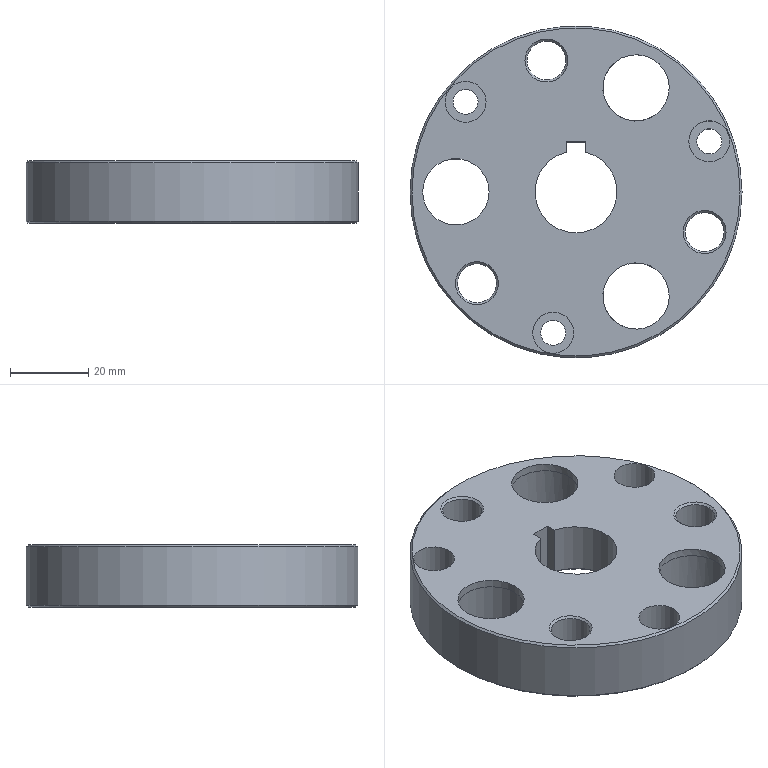Part | NX | features BREP 1 | 1 solid | 45 faces | box 85 x 85 x 16 mm | volume 64345 mm3 | cylinder 18 | cone 15 | plane 12 | commonest cylinder face diameters 6.4 x3 10 x3 10.5 x3 17 x3 19 x3 21 x1
STEP:
#1=CARTESIAN_POINT('',(25.38,26.639,0.));
#2=VERTEX_POINT('',#1);
#3=CARTESIAN_POINT('',(15.38,26.639,0.));
#4=DIRECTION('',(0.,0.,1.));
#5=DIRECTION('',(1.,0.,0.));
#6=AXIS2_PLACEMENT_3D('',#3,#4,#5);
#7=CIRCLE('',#6,10.);
#8=EDGE_CURVE('',#2,#2,#7,.T.);
#9=ORIENTED_EDGE('',*,*,#8,.F.);
#10=EDGE_LOOP('',(#9));
#11=FACE_BOUND('',#10,.T.);
#12=CARTESIAN_POINT('',(24.88,26.639,0.5));
#13=VERTEX_POINT('',#12);
#14=CARTESIAN_POINT('',(15.38,26.639,0.5));
#15=DIRECTION('',(0.,0.,-1.));
#16=DIRECTION('',(1.,0.,0.));
#17=AXIS2_PLACEMENT_3D('',#14,#15,#16);
#18=CIRCLE('',#17,9.5);
#19=EDGE_CURVE('',#13,#13,#18,.T.);
#20=ORIENTED_EDGE('',*,*,#19,.F.);
#21=EDGE_LOOP('',(#20));
#22=FACE_BOUND('',#21,.T.);
#23=CARTESIAN_POINT('',(15.38,26.639,0.));
#24=DIRECTION('',(0.,0.,-1.));
#25=DIRECTION('',(-1.,0.,0.));
#26=AXIS2_PLACEMENT_3D('',#23,#24,#25);
#27=CONICAL_SURFACE('',#26,10.,0.7854);
#28=ADVANCED_FACE('',(#11,#22),#27,.F.);
#29=CARTESIAN_POINT('',(25.38,-26.639,0.));
#30=VERTEX_POINT('',#29);
#31=CARTESIAN_POINT('',(15.38,-26.639,0.));
#32=DIRECTION('',(0.,0.,1.));
#33=DIRECTION('',(1.,0.,0.));
#34=AXIS2_PLACEMENT_3D('',#31,#32,#33);
#35=CIRCLE('',#34,10.);
#36=EDGE_CURVE('',#30,#30,#35,.T.);
#37=ORIENTED_EDGE('',*,*,#36,.F.);
#38=EDGE_LOOP('',(#37));
#39=FACE_BOUND('',#38,.T.);
#40=CARTESIAN_POINT('',(24.88,-26.639,0.5));
#41=VERTEX_POINT('',#40);
#42=CARTESIAN_POINT('',(15.38,-26.639,0.5));
#43=DIRECTION('',(0.,0.,-1.));
#44=DIRECTION('',(1.,0.,0.));
#45=AXIS2_PLACEMENT_3D('',#42,#43,#44);
#46=CIRCLE('',#45,9.5);
#47=EDGE_CURVE('',#41,#41,#46,.T.);
#48=ORIENTED_EDGE('',*,*,#47,.F.);
#49=EDGE_LOOP('',(#48));
#50=FACE_BOUND('',#49,.T.);
#51=CARTESIAN_POINT('',(15.38,-26.639,0.));
#52=DIRECTION('',(0.,0.,-1.));
#53=DIRECTION('',(-1.,0.,0.));
#54=AXIS2_PLACEMENT_3D('',#51,#52,#53);
#55=CONICAL_SURFACE('',#54,10.,0.7854);
#56=ADVANCED_FACE('',(#39,#50),#55,.F.);
#57=CARTESIAN_POINT('',(-20.76,0.,0.));
#58=VERTEX_POINT('',#57);
#59=CARTESIAN_POINT('',(-30.76,0.,0.));
#60=DIRECTION('',(0.,0.,1.));
#61=DIRECTION('',(1.,0.,0.));
#62=AXIS2_PLACEMENT_3D('',#59,#60,#61);
#63=CIRCLE('',#62,10.);
#64=EDGE_CURVE('',#58,#58,#63,.T.);
#65=ORIENTED_EDGE('',*,*,#64,.F.);
#66=EDGE_LOOP('',(#65));
#67=FACE_BOUND('',#66,.T.);
#68=CARTESIAN_POINT('',(-21.26,0.,0.5));
#69=VERTEX_POINT('',#68);
#70=CARTESIAN_POINT('',(-30.76,0.,0.5));
#71=DIRECTION('',(0.,0.,-1.));
#72=DIRECTION('',(1.,0.,0.));
#73=AXIS2_PLACEMENT_3D('',#70,#71,#72);
#74=CIRCLE('',#73,9.5);
#75=EDGE_CURVE('',#69,#69,#74,.T.);
#76=ORIENTED_EDGE('',*,*,#75,.F.);
#77=EDGE_LOOP('',(#76));
#78=FACE_BOUND('',#77,.T.);
#79=CARTESIAN_POINT('',(-30.76,0.,0.));
#80=DIRECTION('',(0.,0.,-1.));
#81=DIRECTION('',(-1.,0.,0.));
#82=AXIS2_PLACEMENT_3D('',#79,#80,#81);
#83=CONICAL_SURFACE('',#82,10.,0.7854);
#84=ADVANCED_FACE('',(#67,#78),#83,.F.);
#85=CARTESIAN_POINT('',(14.5,0.,0.));
#86=VERTEX_POINT('',#85);
#87=CARTESIAN_POINT('',(0.,0.,0.));
#88=DIRECTION('',(0.,0.,1.));
#89=DIRECTION('',(1.,0.,0.));
#90=AXIS2_PLACEMENT_3D('',#87,#88,#89);
#91=CIRCLE('',#90,14.5);
#92=EDGE_CURVE('',#86,#86,#91,.T.);
#93=ORIENTED_EDGE('',*,*,#92,.F.);
#94=EDGE_LOOP('',(#93));
#95=FACE_BOUND('',#94,.T.);
#96=CARTESIAN_POINT('',(14.,0.,0.5));
#97=VERTEX_POINT('',#96);
#98=CARTESIAN_POINT('',(0.,0.,0.5));
#99=DIRECTION('',(0.,0.,-1.));
#100=DIRECTION('',(1.,0.,0.));
#101=AXIS2_PLACEMENT_3D('',#98,#99,#100);
#102=CIRCLE('',#101,14.);
#103=EDGE_CURVE('',#97,#97,#102,.T.);
#104=ORIENTED_EDGE('',*,*,#103,.F.);
#105=EDGE_LOOP('',(#104));
#106=FACE_BOUND('',#105,.T.);
#107=CARTESIAN_POINT('',(0.,0.,0.5));
#108=DIRECTION('',(0.,0.,-1.));
#109=DIRECTION('',(-1.,0.,0.));
#110=AXIS2_PLACEMENT_3D('',#107,#108,#109);
#111=CONICAL_SURFACE('',#110,14.,0.7854);
#112=ADVANCED_FACE('',(#95,#106),#111,.F.);
#113=CARTESIAN_POINT('',(-23.029,23.076,16.));
#114=VERTEX_POINT('',#113);
#115=CARTESIAN_POINT('',(-28.279,23.076,16.));
#116=DIRECTION('',(0.,0.,1.));
#117=DIRECTION('',(1.,0.,0.));
#118=AXIS2_PLACEMENT_3D('',#115,#116,#117);
#119=CIRCLE('',#118,5.25);
#120=EDGE_CURVE('',#114,#114,#119,.T.);
#121=ORIENTED_EDGE('',*,*,#120,.T.);
#122=EDGE_LOOP('',(#121));
#123=FACE_BOUND('',#122,.T.);
#124=CARTESIAN_POINT('',(-23.029,23.076,8.5));
#125=VERTEX_POINT('',#124);
#126=CARTESIAN_POINT('',(-28.279,23.076,8.5));
#127=DIRECTION('',(0.,0.,1.));
#128=DIRECTION('',(1.,0.,0.));
#129=AXIS2_PLACEMENT_3D('',#126,#127,#128);
#130=CIRCLE('',#129,5.25);
#131=EDGE_CURVE('',#125,#125,#130,.T.);
#132=ORIENTED_EDGE('',*,*,#131,.F.);
#133=EDGE_LOOP('',(#132));
#134=FACE_BOUND('',#133,.T.);
#135=CARTESIAN_POINT('',(-28.279,23.076,16.));
#136=DIRECTION('',(0.,0.,1.));
#137=DIRECTION('',(1.,0.,0.));
#138=AXIS2_PLACEMENT_3D('',#135,#136,#137);
#139=CYLINDRICAL_SURFACE('',#138,5.25);
#140=ADVANCED_FACE('',(#123,#134),#139,.F.);
#141=CARTESIAN_POINT('',(39.375,12.952,16.));
#142=VERTEX_POINT('',#141);
#143=CARTESIAN_POINT('',(34.125,12.952,16.));
#144=DIRECTION('',(0.,0.,1.));
#145=DIRECTION('',(1.,0.,0.));
#146=AXIS2_PLACEMENT_3D('',#143,#144,#145);
#147=CIRCLE('',#146,5.25);
#148=EDGE_CURVE('',#142,#142,#147,.T.);
#149=ORIENTED_EDGE('',*,*,#148,.T.);
#150=EDGE_LOOP('',(#149));
#151=FACE_BOUND('',#150,.T.);
#152=CARTESIAN_POINT('',(39.375,12.952,8.5));
#153=VERTEX_POINT('',#152);
#154=CARTESIAN_POINT('',(34.125,12.952,8.5));
#155=DIRECTION('',(0.,0.,1.));
#156=DIRECTION('',(1.,0.,0.));
#157=AXIS2_PLACEMENT_3D('',#154,#155,#156);
#158=CIRCLE('',#157,5.25);
#159=EDGE_CURVE('',#153,#153,#158,.T.);
#160=ORIENTED_EDGE('',*,*,#159,.F.);
#161=EDGE_LOOP('',(#160));
#162=FACE_BOUND('',#161,.T.);
#163=CARTESIAN_POINT('',(34.125,12.952,16.));
#164=DIRECTION('',(0.,0.,1.));
#165=DIRECTION('',(1.,0.,0.));
#166=AXIS2_PLACEMENT_3D('',#163,#164,#165);
#167=CYLINDRICAL_SURFACE('',#166,5.25);
#168=ADVANCED_FACE('',(#151,#162),#167,.F.);
#169=CARTESIAN_POINT('',(-0.5951,-36.029,16.));
#170=VERTEX_POINT('',#169);
#171=CARTESIAN_POINT('',(-5.845,-36.029,16.));
#172=DIRECTION('',(0.,0.,1.));
#173=DIRECTION('',(1.,0.,0.));
#174=AXIS2_PLACEMENT_3D('',#171,#172,#173);
#175=CIRCLE('',#174,5.25);
#176=EDGE_CURVE('',#170,#170,#175,.T.);
#177=ORIENTED_EDGE('',*,*,#176,.T.);
#178=EDGE_LOOP('',(#177));
#179=FACE_BOUND('',#178,.T.);
#180=CARTESIAN_POINT('',(-0.5951,-36.029,8.5));
#181=VERTEX_POINT('',#180);
#182=CARTESIAN_POINT('',(-5.845,-36.029,8.5));
#183=DIRECTION('',(0.,0.,1.));
#184=DIRECTION('',(1.,0.,0.));
#185=AXIS2_PLACEMENT_3D('',#182,#183,#184);
#186=CIRCLE('',#185,5.25);
#187=EDGE_CURVE('',#181,#181,#186,.T.);
#188=ORIENTED_EDGE('',*,*,#187,.F.);
#189=EDGE_LOOP('',(#188));
#190=FACE_BOUND('',#189,.T.);
#191=CARTESIAN_POINT('',(-5.845,-36.029,16.));
#192=DIRECTION('',(0.,0.,1.));
#193=DIRECTION('',(1.,0.,0.));
#194=AXIS2_PLACEMENT_3D('',#191,#192,#193);
#195=CYLINDRICAL_SURFACE('',#194,5.25);
#196=ADVANCED_FACE('',(#179,#190),#195,.F.);
#197=ORIENTED_EDGE('',*,*,#103,.T.);
#198=EDGE_LOOP('',(#197));
#199=FACE_BOUND('',#198,.T.);
#200=CARTESIAN_POINT('',(-14.,0.,3.));
#201=VERTEX_POINT('',#200);
#202=CARTESIAN_POINT('',(0.,0.,3.));
#203=DIRECTION('',(0.,0.,-1.));
#204=DIRECTION('',(-1.,0.,0.));
#205=AXIS2_PLACEMENT_3D('',#202,#203,#204);
#206=CIRCLE('',#205,14.);
#207=EDGE_CURVE('',#201,#201,#206,.T.);
#208=ORIENTED_EDGE('',*,*,#207,.F.);
#209=EDGE_LOOP('',(#208));
#210=FACE_BOUND('',#209,.T.);
#211=CARTESIAN_POINT('',(0.,0.,3.));
#212=DIRECTION('',(0.,0.,-1.));
#213=DIRECTION('',(-1.,0.,0.));
#214=AXIS2_PLACEMENT_3D('',#211,#212,#213);
#215=CYLINDRICAL_SURFACE('',#214,14.);
#216=ADVANCED_FACE('',(#199,#210),#215,.F.);
#217=CARTESIAN_POINT('',(42.5,0.,15.5));
#218=VERTEX_POINT('',#217);
#219=CARTESIAN_POINT('',(0.,0.,15.5));
#220=DIRECTION('',(0.,0.,-1.));
#221=DIRECTION('',(1.,0.,0.));
#222=AXIS2_PLACEMENT_3D('',#219,#220,#221);
#223=CIRCLE('',#222,42.5);
#224=EDGE_CURVE('',#218,#218,#223,.T.);
#225=ORIENTED_EDGE('',*,*,#224,.F.);
#226=EDGE_LOOP('',(#225));
#227=FACE_BOUND('',#226,.T.);
#228=CARTESIAN_POINT('',(42.,0.,16.));
#229=VERTEX_POINT('',#228);
#230=CARTESIAN_POINT('',(0.,0.,16.));
#231=DIRECTION('',(0.,0.,1.));
#232=DIRECTION('',(1.,0.,0.));
#233=AXIS2_PLACEMENT_3D('',#230,#231,#232);
#234=CIRCLE('',#233,42.);
#235=EDGE_CURVE('',#229,#229,#234,.T.);
#236=ORIENTED_EDGE('',*,*,#235,.F.);
#237=EDGE_LOOP('',(#236));
#238=FACE_BOUND('',#237,.T.);
#239=CARTESIAN_POINT('',(0.,0.,16.));
#240=DIRECTION('',(0.,0.,-1.));
#241=DIRECTION('',(-1.,0.,0.));
#242=AXIS2_PLACEMENT_3D('',#239,#240,#241);
#243=CONICAL_SURFACE('',#242,42.,0.7854);
#244=ADVANCED_FACE('',(#227,#238),#243,.T.);
#245=CARTESIAN_POINT('',(42.5,0.,0.5));
#246=VERTEX_POINT('',#245);
#247=CARTESIAN_POINT('',(0.,0.,0.5));
#248=DIRECTION('',(0.,0.,1.));
#249=DIRECTION('',(1.,0.,0.));
#250=AXIS2_PLACEMENT_3D('',#247,#248,#249);
#251=CIRCLE('',#250,42.5);
#252=EDGE_CURVE('',#246,#246,#251,.T.);
#253=ORIENTED_EDGE('',*,*,#252,.F.);
#254=EDGE_LOOP('',(#253));
#255=FACE_BOUND('',#254,.T.);
#256=CARTESIAN_POINT('',(42.,0.,0.));
#257=VERTEX_POINT('',#256);
#258=CARTESIAN_POINT('',(0.,0.,0.));
#259=DIRECTION('',(0.,0.,-1.));
#260=DIRECTION('',(1.,0.,0.));
#261=AXIS2_PLACEMENT_3D('',#258,#259,#260);
#262=CIRCLE('',#261,42.);
#263=EDGE_CURVE('',#257,#257,#262,.T.);
#264=ORIENTED_EDGE('',*,*,#263,.F.);
#265=EDGE_LOOP('',(#264));
#266=FACE_BOUND('',#265,.T.);
#267=CARTESIAN_POINT('',(0.,0.,0.5));
#268=DIRECTION('',(0.,0.,1.));
#269=DIRECTION('',(1.,0.,0.));
#270=AXIS2_PLACEMENT_3D('',#267,#268,#269);
#271=CONICAL_SURFACE('',#270,42.5,0.7854);
#272=ADVANCED_FACE('',(#255,#266),#271,.T.);
#273=CARTESIAN_POINT('',(38.427,-10.265,16.));
#274=VERTEX_POINT('',#273);
#275=CARTESIAN_POINT('',(32.927,-10.265,16.));
#276=DIRECTION('',(0.,0.,-1.));
#277=DIRECTION('',(1.,0.,0.));
#278=AXIS2_PLACEMENT_3D('',#275,#276,#277);
#279=CIRCLE('',#278,5.5);
#280=EDGE_CURVE('',#274,#274,#279,.T.);
#281=ORIENTED_EDGE('',*,*,#280,.F.);
#282=EDGE_LOOP('',(#281));
#283=FACE_BOUND('',#282,.T.);
#284=CARTESIAN_POINT('',(37.927,-10.265,15.5));
#285=VERTEX_POINT('',#284);
#286=CARTESIAN_POINT('',(32.927,-10.265,15.5));
#287=DIRECTION('',(0.,0.,1.));
#288=DIRECTION('',(1.,0.,0.));
#289=AXIS2_PLACEMENT_3D('',#286,#287,#288);
#290=CIRCLE('',#289,5.);
#291=EDGE_CURVE('',#285,#285,#290,.T.);
#292=ORIENTED_EDGE('',*,*,#291,.F.);
#293=EDGE_LOOP('',(#292));
#294=FACE_BOUND('',#293,.T.);
#295=CARTESIAN_POINT('',(32.927,-10.265,16.));
#296=DIRECTION('',(0.,0.,1.));
#297=DIRECTION('',(1.,0.,0.));
#298=AXIS2_PLACEMENT_3D('',#295,#296,#297);
#299=CONICAL_SURFACE('',#298,5.5,0.7854);
#300=ADVANCED_FACE('',(#283,#294),#299,.F.);
#301=CARTESIAN_POINT('',(38.427,-10.265,0.));
#302=VERTEX_POINT('',#301);
#303=CARTESIAN_POINT('',(32.927,-10.265,0.));
#304=DIRECTION('',(0.,0.,1.));
#305=DIRECTION('',(1.,0.,0.));
#306=AXIS2_PLACEMENT_3D('',#303,#304,#305);
#307=CIRCLE('',#306,5.5);
#308=EDGE_CURVE('',#302,#302,#307,.T.);
#309=ORIENTED_EDGE('',*,*,#308,.F.);
#310=EDGE_LOOP('',(#309));
#311=FACE_BOUND('',#310,.T.);
#312=CARTESIAN_POINT('',(37.927,-10.265,0.5));
#313=VERTEX_POINT('',#312);
#314=CARTESIAN_POINT('',(32.927,-10.265,0.5));
#315=DIRECTION('',(0.,0.,-1.));
#316=DIRECTION('',(1.,0.,0.));
#317=AXIS2_PLACEMENT_3D('',#314,#315,#316);
#318=CIRCLE('',#317,5.);
#319=EDGE_CURVE('',#313,#313,#318,.T.);
#320=ORIENTED_EDGE('',*,*,#319,.F.);
#321=EDGE_LOOP('',(#320));
#322=FACE_BOUND('',#321,.T.);
#323=CARTESIAN_POINT('',(32.927,-10.265,0.5));
#324=DIRECTION('',(0.,0.,-1.));
#325=DIRECTION('',(-1.,0.,0.));
#326=AXIS2_PLACEMENT_3D('',#323,#324,#325);
#327=CONICAL_SURFACE('',#326,5.,0.7854);
#328=ADVANCED_FACE('',(#311,#322),#327,.F.);
#329=CARTESIAN_POINT('',(37.825,12.952,0.));
#330=VERTEX_POINT('',#329);
#331=CARTESIAN_POINT('',(34.125,12.952,0.));
#332=DIRECTION('',(0.,0.,1.));
#333=DIRECTION('',(1.,0.,0.));
#334=AXIS2_PLACEMENT_3D('',#331,#332,#333);
#335=CIRCLE('',#334,3.7);
#336=EDGE_CURVE('',#330,#330,#335,.T.);
#337=ORIENTED_EDGE('',*,*,#336,.F.);
#338=EDGE_LOOP('',(#337));
#339=FACE_BOUND('',#338,.T.);
#340=CARTESIAN_POINT('',(37.325,12.952,0.5));
#341=VERTEX_POINT('',#340);
#342=CARTESIAN_POINT('',(34.125,12.952,0.5));
#343=DIRECTION('',(0.,0.,-1.));
#344=DIRECTION('',(1.,0.,0.));
#345=AXIS2_PLACEMENT_3D('',#342,#343,#344);
#346=CIRCLE('',#345,3.2);
#347=EDGE_CURVE('',#341,#341,#346,.T.);
#348=ORIENTED_EDGE('',*,*,#347,.F.);
#349=EDGE_LOOP('',(#348));
#350=FACE_BOUND('',#349,.T.);
#351=CARTESIAN_POINT('',(34.125,12.952,0.5));
#352=DIRECTION('',(0.,0.,-1.));
#353=DIRECTION('',(-1.,0.,0.));
#354=AXIS2_PLACEMENT_3D('',#351,#352,#353);
#355=CONICAL_SURFACE('',#354,3.2,0.7854);
#356=ADVANCED_FACE('',(#339,#350),#355,.F.);
#357=CARTESIAN_POINT('',(-2.074,33.648,16.));
#358=VERTEX_POINT('',#357);
#359=CARTESIAN_POINT('',(-7.574,33.648,16.));
#360=DIRECTION('',(0.,0.,-1.));
#361=DIRECTION('',(1.,0.,0.));
#362=AXIS2_PLACEMENT_3D('',#359,#360,#361);
#363=CIRCLE('',#362,5.5);
#364=EDGE_CURVE('',#358,#358,#363,.T.);
#365=ORIENTED_EDGE('',*,*,#364,.F.);
#366=EDGE_LOOP('',(#365));
#367=FACE_BOUND('',#366,.T.);
#368=CARTESIAN_POINT('',(-2.574,33.648,15.5));
#369=VERTEX_POINT('',#368);
#370=CARTESIAN_POINT('',(-7.574,33.648,15.5));
#371=DIRECTION('',(0.,0.,1.));
#372=DIRECTION('',(1.,0.,0.));
#373=AXIS2_PLACEMENT_3D('',#370,#371,#372);
#374=CIRCLE('',#373,5.);
#375=EDGE_CURVE('',#369,#369,#374,.T.);
#376=ORIENTED_EDGE('',*,*,#375,.F.);
#377=EDGE_LOOP('',(#376));
#378=FACE_BOUND('',#377,.T.);
#379=CARTESIAN_POINT('',(-7.574,33.648,16.));
#380=DIRECTION('',(0.,0.,1.));
#381=DIRECTION('',(1.,0.,0.));
#382=AXIS2_PLACEMENT_3D('',#379,#380,#381);
#383=CONICAL_SURFACE('',#382,5.5,0.7854);
#384=ADVANCED_FACE('',(#367,#378),#383,.F.);
#385=CARTESIAN_POINT('',(-2.074,33.648,0.));
#386=VERTEX_POINT('',#385);
#387=CARTESIAN_POINT('',(-7.574,33.648,0.));
#388=DIRECTION('',(0.,0.,1.));
#389=DIRECTION('',(1.,0.,0.));
#390=AXIS2_PLACEMENT_3D('',#387,#388,#389);
#391=CIRCLE('',#390,5.5);
#392=EDGE_CURVE('',#386,#386,#391,.T.);
#393=ORIENTED_EDGE('',*,*,#392,.F.);
#394=EDGE_LOOP('',(#393));
#395=FACE_BOUND('',#394,.T.);
#396=CARTESIAN_POINT('',(-2.574,33.648,0.5));
#397=VERTEX_POINT('',#396);
#398=CARTESIAN_POINT('',(-7.574,33.648,0.5));
#399=DIRECTION('',(0.,0.,-1.));
#400=DIRECTION('',(1.,0.,0.));
#401=AXIS2_PLACEMENT_3D('',#398,#399,#400);
#402=CIRCLE('',#401,5.);
#403=EDGE_CURVE('',#397,#397,#402,.T.);
#404=ORIENTED_EDGE('',*,*,#403,.F.);
#405=EDGE_LOOP('',(#404));
#406=FACE_BOUND('',#405,.T.);
#407=CARTESIAN_POINT('',(-7.574,33.648,0.5));
#408=DIRECTION('',(0.,0.,-1.));
#409=DIRECTION('',(-1.,0.,0.));
#410=AXIS2_PLACEMENT_3D('',#407,#408,#409);
#411=CONICAL_SURFACE('',#410,5.,0.7854);
#412=ADVANCED_FACE('',(#395,#406),#411,.F.);
#413=CARTESIAN_POINT('',(-24.579,23.076,0.));
#414=VERTEX_POINT('',#413);
#415=CARTESIAN_POINT('',(-28.279,23.076,0.));
#416=DIRECTION('',(0.,0.,1.));
#417=DIRECTION('',(1.,0.,0.));
#418=AXIS2_PLACEMENT_3D('',#415,#416,#417);
#419=CIRCLE('',#418,3.7);
#420=EDGE_CURVE('',#414,#414,#419,.T.);
#421=ORIENTED_EDGE('',*,*,#420,.F.);
#422=EDGE_LOOP('',(#421));
#423=FACE_BOUND('',#422,.T.);
#424=CARTESIAN_POINT('',(-25.079,23.076,0.5));
#425=VERTEX_POINT('',#424);
#426=CARTESIAN_POINT('',(-28.279,23.076,0.5));
#427=DIRECTION('',(0.,0.,-1.));
#428=DIRECTION('',(1.,0.,0.));
#429=AXIS2_PLACEMENT_3D('',#426,#427,#428);
#430=CIRCLE('',#429,3.2);
#431=EDGE_CURVE('',#425,#425,#430,.T.);
#432=ORIENTED_EDGE('',*,*,#431,.F.);
#433=EDGE_LOOP('',(#432));
#434=FACE_BOUND('',#433,.T.);
#435=CARTESIAN_POINT('',(-28.279,23.076,0.5));
#436=DIRECTION('',(0.,0.,-1.));
#437=DIRECTION('',(-1.,0.,0.));
#438=AXIS2_PLACEMENT_3D('',#435,#436,#437);
#439=CONICAL_SURFACE('',#438,3.2,0.7854);
#440=ADVANCED_FACE('',(#423,#434),#439,.F.);
#441=ORIENTED_EDGE('',*,*,#47,.T.);
#442=EDGE_LOOP('',(#441));
#443=FACE_BOUND('',#442,.T.);
#444=CARTESIAN_POINT('',(10.63,-18.412,14.));
#445=VERTEX_POINT('',#444);
#446=CARTESIAN_POINT('',(15.38,-26.639,14.));
#447=DIRECTION('',(0.,0.,1.));
#448=DIRECTION('',(-0.5,0.866,0.));
#449=AXIS2_PLACEMENT_3D('',#446,#447,#448);
#450=CIRCLE('',#449,9.5);
#451=EDGE_CURVE('',#445,#445,#450,.T.);
#452=ORIENTED_EDGE('',*,*,#451,.T.);
#453=EDGE_LOOP('',(#452));
#454=FACE_BOUND('',#453,.T.);
#455=CARTESIAN_POINT('',(15.38,-26.639,14.));
#456=DIRECTION('',(0.,0.,-1.));
#457=DIRECTION('',(-1.,0.,0.));
#458=AXIS2_PLACEMENT_3D('',#455,#456,#457);
#459=CYLINDRICAL_SURFACE('',#458,9.5);
#460=ADVANCED_FACE('',(#443,#454),#459,.F.);
#461=ORIENTED_EDGE('',*,*,#19,.T.);
#462=EDGE_LOOP('',(#461));
#463=FACE_BOUND('',#462,.T.);
#464=CARTESIAN_POINT('',(10.63,18.412,14.));
#465=VERTEX_POINT('',#464);
#466=CARTESIAN_POINT('',(15.38,26.639,14.));
#467=DIRECTION('',(0.,0.,1.));
#468=DIRECTION('',(-0.5,-0.866,0.));
#469=AXIS2_PLACEMENT_3D('',#466,#467,#468);
#470=CIRCLE('',#469,9.5);
#471=EDGE_CURVE('',#465,#465,#470,.T.);
#472=ORIENTED_EDGE('',*,*,#471,.T.);
#473=EDGE_LOOP('',(#472));
#474=FACE_BOUND('',#473,.T.);
#475=CARTESIAN_POINT('',(15.38,26.639,14.));
#476=DIRECTION('',(0.,0.,-1.));
#477=DIRECTION('',(-1.,0.,0.));
#478=AXIS2_PLACEMENT_3D('',#475,#476,#477);
#479=CYLINDRICAL_SURFACE('',#478,9.5);
#480=ADVANCED_FACE('',(#463,#474),#479,.F.);
#481=ORIENTED_EDGE('',*,*,#347,.T.);
#482=EDGE_LOOP('',(#481));
#483=FACE_BOUND('',#482,.T.);
#484=CARTESIAN_POINT('',(37.325,12.952,8.5));
#485=VERTEX_POINT('',#484);
#486=CARTESIAN_POINT('',(34.125,12.952,8.5));
#487=DIRECTION('',(0.,0.,1.));
#488=DIRECTION('',(1.,0.,0.));
#489=AXIS2_PLACEMENT_3D('',#486,#487,#488);
#490=CIRCLE('',#489,3.2);
#491=EDGE_CURVE('',#485,#485,#490,.T.);
#492=ORIENTED_EDGE('',*,*,#491,.T.);
#493=EDGE_LOOP('',(#492));
#494=FACE_BOUND('',#493,.T.);
#495=CARTESIAN_POINT('',(34.125,12.952,16.));
#496=DIRECTION('',(0.,0.,-1.));
#497=DIRECTION('',(-1.,0.,0.));
#498=AXIS2_PLACEMENT_3D('',#495,#496,#497);
#499=CYLINDRICAL_SURFACE('',#498,3.2);
#500=ADVANCED_FACE('',(#483,#494),#499,.F.);
#501=ORIENTED_EDGE('',*,*,#319,.T.);
#502=EDGE_LOOP('',(#501));
#503=FACE_BOUND('',#502,.T.);
#504=ORIENTED_EDGE('',*,*,#291,.T.);
#505=EDGE_LOOP('',(#504));
#506=FACE_BOUND('',#505,.T.);
#507=CARTESIAN_POINT('',(32.927,-10.265,16.));
#508=DIRECTION('',(0.,0.,-1.));
#509=DIRECTION('',(-1.,0.,0.));
#510=AXIS2_PLACEMENT_3D('',#507,#508,#509);
#511=CYLINDRICAL_SURFACE('',#510,5.);
#512=ADVANCED_FACE('',(#503,#506),#511,.F.);
#513=CARTESIAN_POINT('',(23.88,-26.639,14.));
#514=VERTEX_POINT('',#513);
#515=CARTESIAN_POINT('',(15.38,-26.639,14.));
#516=DIRECTION('',(0.,0.,-1.));
#517=DIRECTION('',(1.,0.,0.));
#518=AXIS2_PLACEMENT_3D('',#515,#516,#517);
#519=CIRCLE('',#518,8.5);
#520=EDGE_CURVE('',#514,#514,#519,.T.);
#521=ORIENTED_EDGE('',*,*,#520,.T.);
#522=EDGE_LOOP('',(#521));
#523=FACE_BOUND('',#522,.T.);
#524=CARTESIAN_POINT('',(19.63,-34.,16.));
#525=VERTEX_POINT('',#524);
#526=CARTESIAN_POINT('',(15.38,-26.639,16.));
#527=DIRECTION('',(0.,0.,-1.));
#528=DIRECTION('',(0.5,-0.866,0.));
#529=AXIS2_PLACEMENT_3D('',#526,#527,#528);
#530=CIRCLE('',#529,8.5);
#531=EDGE_CURVE('',#525,#525,#530,.T.);
#532=ORIENTED_EDGE('',*,*,#531,.F.);
#533=EDGE_LOOP('',(#532));
#534=FACE_BOUND('',#533,.T.);
#535=CARTESIAN_POINT('',(15.38,-26.639,16.));
#536=DIRECTION('',(0.,0.,-1.));
#537=DIRECTION('',(-1.,0.,0.));
#538=AXIS2_PLACEMENT_3D('',#535,#536,#537);
#539=CYLINDRICAL_SURFACE('',#538,8.5);
#540=ADVANCED_FACE('',(#523,#534),#539,.F.);
#541=ORIENTED_EDGE('',*,*,#431,.T.);
#542=EDGE_LOOP('',(#541));
#543=FACE_BOUND('',#542,.T.);
#544=CARTESIAN_POINT('',(-25.079,23.076,8.5));
#545=VERTEX_POINT('',#544);
#546=CARTESIAN_POINT('',(-28.279,23.076,8.5));
#547=DIRECTION('',(0.,0.,1.));
#548=DIRECTION('',(1.,0.,0.));
#549=AXIS2_PLACEMENT_3D('',#546,#547,#548);
#550=CIRCLE('',#549,3.2);
#551=EDGE_CURVE('',#545,#545,#550,.T.);
#552=ORIENTED_EDGE('',*,*,#551,.T.);
#553=EDGE_LOOP('',(#552));
#554=FACE_BOUND('',#553,.T.);
#555=CARTESIAN_POINT('',(-28.279,23.076,16.));
#556=DIRECTION('',(0.,0.,-1.));
#557=DIRECTION('',(-1.,0.,0.));
#558=AXIS2_PLACEMENT_3D('',#555,#556,#557);
#559=CYLINDRICAL_SURFACE('',#558,3.2);
#560=ADVANCED_FACE('',(#543,#554),#559,.F.);
#561=ORIENTED_EDGE('',*,*,#403,.T.);
#562=EDGE_LOOP('',(#561));
#563=FACE_BOUND('',#562,.T.);
#564=ORIENTED_EDGE('',*,*,#375,.T.);
#565=EDGE_LOOP('',(#564));
#566=FACE_BOUND('',#565,.T.);
#567=CARTESIAN_POINT('',(-7.574,33.648,16.));
#568=DIRECTION('',(0.,0.,-1.));
#569=DIRECTION('',(-1.,0.,0.));
#570=AXIS2_PLACEMENT_3D('',#567,#568,#569);
#571=CYLINDRICAL_SURFACE('',#570,5.);
#572=ADVANCED_FACE('',(#563,#566),#571,.F.);
#573=CARTESIAN_POINT('',(23.88,26.639,14.));
#574=VERTEX_POINT('',#573);
#575=CARTESIAN_POINT('',(15.38,26.639,14.));
#576=DIRECTION('',(0.,0.,-1.));
#577=DIRECTION('',(1.,0.,0.));
#578=AXIS2_PLACEMENT_3D('',#575,#576,#577);
#579=CIRCLE('',#578,8.5);
#580=EDGE_CURVE('',#574,#574,#579,.T.);
#581=ORIENTED_EDGE('',*,*,#580,.T.);
#582=EDGE_LOOP('',(#581));
#583=FACE_BOUND('',#582,.T.);
#584=CARTESIAN_POINT('',(19.63,34.,16.));
#585=VERTEX_POINT('',#584);
#586=CARTESIAN_POINT('',(15.38,26.639,16.));
#587=DIRECTION('',(0.,0.,-1.));
#588=DIRECTION('',(0.5,0.866,0.));
#589=AXIS2_PLACEMENT_3D('',#586,#587,#588);
#590=CIRCLE('',#589,8.5);
#591=EDGE_CURVE('',#585,#585,#590,.T.);
#592=ORIENTED_EDGE('',*,*,#591,.F.);
#593=EDGE_LOOP('',(#592));
#594=FACE_BOUND('',#593,.T.);
#595=CARTESIAN_POINT('',(15.38,26.639,16.));
#596=DIRECTION('',(0.,0.,-1.));
#597=DIRECTION('',(-1.,0.,0.));
#598=AXIS2_PLACEMENT_3D('',#595,#596,#597);
#599=CYLINDRICAL_SURFACE('',#598,8.5);
#600=ADVANCED_FACE('',(#583,#594),#599,.F.);
#601=CARTESIAN_POINT('',(-19.853,-23.383,16.));
#602=VERTEX_POINT('',#601);
#603=CARTESIAN_POINT('',(-25.353,-23.383,16.));
#604=DIRECTION('',(0.,0.,-1.));
#605=DIRECTION('',(1.,0.,0.));
#606=AXIS2_PLACEMENT_3D('',#603,#604,#605);
#607=CIRCLE('',#606,5.5);
#608=EDGE_CURVE('',#602,#602,#607,.T.);
#609=ORIENTED_EDGE('',*,*,#608,.F.);
#610=EDGE_LOOP('',(#609));
#611=FACE_BOUND('',#610,.T.);
#612=CARTESIAN_POINT('',(-20.353,-23.383,15.5));
#613=VERTEX_POINT('',#612);
#614=CARTESIAN_POINT('',(-25.353,-23.383,15.5));
#615=DIRECTION('',(0.,0.,1.));
#616=DIRECTION('',(1.,0.,0.));
#617=AXIS2_PLACEMENT_3D('',#614,#615,#616);
#618=CIRCLE('',#617,5.);
#619=EDGE_CURVE('',#613,#613,#618,.T.);
#620=ORIENTED_EDGE('',*,*,#619,.F.);
#621=EDGE_LOOP('',(#620));
#622=FACE_BOUND('',#621,.T.);
#623=CARTESIAN_POINT('',(-25.353,-23.383,16.));
#624=DIRECTION('',(0.,0.,1.));
#625=DIRECTION('',(1.,0.,0.));
#626=AXIS2_PLACEMENT_3D('',#623,#624,#625);
#627=CONICAL_SURFACE('',#626,5.5,0.7854);
#628=ADVANCED_FACE('',(#611,#622),#627,.F.);
#629=CARTESIAN_POINT('',(-19.853,-23.383,0.));
#630=VERTEX_POINT('',#629);
#631=CARTESIAN_POINT('',(-25.353,-23.383,0.));
#632=DIRECTION('',(0.,0.,1.));
#633=DIRECTION('',(1.,0.,0.));
#634=AXIS2_PLACEMENT_3D('',#631,#632,#633);
#635=CIRCLE('',#634,5.5);
#636=EDGE_CURVE('',#630,#630,#635,.T.);
#637=ORIENTED_EDGE('',*,*,#636,.F.);
#638=EDGE_LOOP('',(#637));
#639=FACE_BOUND('',#638,.T.);
#640=CARTESIAN_POINT('',(-20.353,-23.383,0.5));
#641=VERTEX_POINT('',#640);
#642=CARTESIAN_POINT('',(-25.353,-23.383,0.5));
#643=DIRECTION('',(0.,0.,-1.));
#644=DIRECTION('',(1.,0.,0.));
#645=AXIS2_PLACEMENT_3D('',#642,#643,#644);
#646=CIRCLE('',#645,5.);
#647=EDGE_CURVE('',#641,#641,#646,.T.);
#648=ORIENTED_EDGE('',*,*,#647,.F.);
#649=EDGE_LOOP('',(#648));
#650=FACE_BOUND('',#649,.T.);
#651=CARTESIAN_POINT('',(-25.353,-23.383,0.5));
#652=DIRECTION('',(0.,0.,-1.));
#653=DIRECTION('',(-1.,0.,0.));
#654=AXIS2_PLACEMENT_3D('',#651,#652,#653);
#655=CONICAL_SURFACE('',#654,5.,0.7854);
#656=ADVANCED_FACE('',(#639,#650),#655,.F.);
#657=CARTESIAN_POINT('',(-2.145,-36.029,0.));
#658=VERTEX_POINT('',#657);
#659=CARTESIAN_POINT('',(-5.845,-36.029,0.));
#660=DIRECTION('',(0.,0.,1.));
#661=DIRECTION('',(1.,0.,0.));
#662=AXIS2_PLACEMENT_3D('',#659,#660,#661);
#663=CIRCLE('',#662,3.7);
#664=EDGE_CURVE('',#658,#658,#663,.T.);
#665=ORIENTED_EDGE('',*,*,#664,.F.);
#666=EDGE_LOOP('',(#665));
#667=FACE_BOUND('',#666,.T.);
#668=CARTESIAN_POINT('',(-2.645,-36.029,0.5));
#669=VERTEX_POINT('',#668);
#670=CARTESIAN_POINT('',(-5.845,-36.029,0.5));
#671=DIRECTION('',(0.,0.,-1.));
#672=DIRECTION('',(1.,0.,0.));
#673=AXIS2_PLACEMENT_3D('',#670,#671,#672);
#674=CIRCLE('',#673,3.2);
#675=EDGE_CURVE('',#669,#669,#674,.T.);
#676=ORIENTED_EDGE('',*,*,#675,.F.);
#677=EDGE_LOOP('',(#676));
#678=FACE_BOUND('',#677,.T.);
#679=CARTESIAN_POINT('',(-5.845,-36.029,0.5));
#680=DIRECTION('',(0.,0.,-1.));
#681=DIRECTION('',(-1.,0.,0.));
#682=AXIS2_PLACEMENT_3D('',#679,#680,#681);
#683=CONICAL_SURFACE('',#682,3.2,0.7854);
#684=ADVANCED_FACE('',(#667,#678),#683,.F.);
#685=ORIENTED_EDGE('',*,*,#75,.T.);
#686=EDGE_LOOP('',(#685));
#687=FACE_BOUND('',#686,.T.);
#688=CARTESIAN_POINT('',(-21.26,0.,14.));
#689=VERTEX_POINT('',#688);
#690=CARTESIAN_POINT('',(-30.76,0.,14.));
#691=DIRECTION('',(0.,0.,1.));
#692=DIRECTION('',(1.,0.,0.));
#693=AXIS2_PLACEMENT_3D('',#690,#691,#692);
#694=CIRCLE('',#693,9.5);
#695=EDGE_CURVE('',#689,#689,#694,.T.);
#696=ORIENTED_EDGE('',*,*,#695,.T.);
#697=EDGE_LOOP('',(#696));
#698=FACE_BOUND('',#697,.T.);
#699=CARTESIAN_POINT('',(-30.76,0.,14.));
#700=DIRECTION('',(0.,0.,-1.));
#701=DIRECTION('',(-1.,0.,0.));
#702=AXIS2_PLACEMENT_3D('',#699,#700,#701);
#703=CYLINDRICAL_SURFACE('',#702,9.5);
#704=ADVANCED_FACE('',(#687,#698),#703,.F.);
#705=ORIENTED_EDGE('',*,*,#675,.T.);
#706=EDGE_LOOP('',(#705));
#707=FACE_BOUND('',#706,.T.);
#708=CARTESIAN_POINT('',(-2.645,-36.029,8.5));
#709=VERTEX_POINT('',#708);
#710=CARTESIAN_POINT('',(-5.845,-36.029,8.5));
#711=DIRECTION('',(0.,0.,1.));
#712=DIRECTION('',(1.,0.,0.));
#713=AXIS2_PLACEMENT_3D('',#710,#711,#712);
#714=CIRCLE('',#713,3.2);
#715=EDGE_CURVE('',#709,#709,#714,.T.);
#716=ORIENTED_EDGE('',*,*,#715,.T.);
#717=EDGE_LOOP('',(#716));
#718=FACE_BOUND('',#717,.T.);
#719=CARTESIAN_POINT('',(-5.845,-36.029,16.));
#720=DIRECTION('',(0.,0.,-1.));
#721=DIRECTION('',(-1.,0.,0.));
#722=AXIS2_PLACEMENT_3D('',#719,#720,#721);
#723=CYLINDRICAL_SURFACE('',#722,3.2);
#724=ADVANCED_FACE('',(#707,#718),#723,.F.);
#725=ORIENTED_EDGE('',*,*,#647,.T.);
#726=EDGE_LOOP('',(#725));
#727=FACE_BOUND('',#726,.T.);
#728=ORIENTED_EDGE('',*,*,#619,.T.);
#729=EDGE_LOOP('',(#728));
#730=FACE_BOUND('',#729,.T.);
#731=CARTESIAN_POINT('',(-25.353,-23.383,16.));
#732=DIRECTION('',(0.,0.,-1.));
#733=DIRECTION('',(-1.,0.,0.));
#734=AXIS2_PLACEMENT_3D('',#731,#732,#733);
#735=CYLINDRICAL_SURFACE('',#734,5.);
#736=ADVANCED_FACE('',(#727,#730),#735,.F.);
#737=CARTESIAN_POINT('',(-22.26,0.,14.));
#738=VERTEX_POINT('',#737);
#739=CARTESIAN_POINT('',(-30.76,0.,14.));
#740=DIRECTION('',(0.,0.,-1.));
#741=DIRECTION('',(1.,0.,0.));
#742=AXIS2_PLACEMENT_3D('',#739,#740,#741);
#743=CIRCLE('',#742,8.5);
#744=EDGE_CURVE('',#738,#738,#743,.T.);
#745=ORIENTED_EDGE('',*,*,#744,.T.);
#746=EDGE_LOOP('',(#745));
#747=FACE_BOUND('',#746,.T.);
#748=CARTESIAN_POINT('',(-39.26,0.,16.));
#749=VERTEX_POINT('',#748);
#750=CARTESIAN_POINT('',(-30.76,0.,16.));
#751=DIRECTION('',(0.,0.,-1.));
#752=DIRECTION('',(-1.,0.,0.));
#753=AXIS2_PLACEMENT_3D('',#750,#751,#752);
#754=CIRCLE('',#753,8.5);
#755=EDGE_CURVE('',#749,#749,#754,.T.);
#756=ORIENTED_EDGE('',*,*,#755,.F.);
#757=EDGE_LOOP('',(#756));
#758=FACE_BOUND('',#757,.T.);
#759=CARTESIAN_POINT('',(-30.76,0.,16.));
#760=DIRECTION('',(0.,0.,-1.));
#761=DIRECTION('',(-1.,0.,0.));
#762=AXIS2_PLACEMENT_3D('',#759,#760,#761);
#763=CYLINDRICAL_SURFACE('',#762,8.5);
#764=ADVANCED_FACE('',(#747,#758),#763,.F.);
#765=ORIENTED_EDGE('',*,*,#252,.T.);
#766=EDGE_LOOP('',(#765));
#767=FACE_BOUND('',#766,.T.);
#768=ORIENTED_EDGE('',*,*,#224,.T.);
#769=EDGE_LOOP('',(#768));
#770=FACE_BOUND('',#769,.T.);
#771=CARTESIAN_POINT('',(0.,0.,16.));
#772=DIRECTION('',(0.,0.,-1.));
#773=DIRECTION('',(-1.,0.,0.));
#774=AXIS2_PLACEMENT_3D('',#771,#772,#773);
#775=CYLINDRICAL_SURFACE('',#774,42.5);
#776=ADVANCED_FACE('',(#767,#770),#775,.T.);
#777=CARTESIAN_POINT('',(-2.5,10.198,16.));
#778=VERTEX_POINT('',#777);
#779=CARTESIAN_POINT('',(2.5,10.198,16.));
#780=VERTEX_POINT('',#779);
#781=CARTESIAN_POINT('',(0.,0.,16.));
#782=DIRECTION('',(0.,0.,1.));
#783=DIRECTION('',(1.,0.,0.));
#784=AXIS2_PLACEMENT_3D('',#781,#782,#783);
#785=CIRCLE('',#784,10.5);
#786=EDGE_CURVE('',#778,#780,#785,.T.);
#787=ORIENTED_EDGE('',*,*,#786,.T.);
#788=CARTESIAN_POINT('',(2.5,10.198,3.));
#789=VERTEX_POINT('',#788);
#790=CARTESIAN_POINT('',(2.5,10.198,16.));
#791=DIRECTION('',(0.,0.,-1.));
#792=VECTOR('',#791,1000.);
#793=LINE('',#790,#792);
#794=EDGE_CURVE('',#780,#789,#793,.T.);
#795=ORIENTED_EDGE('',*,*,#794,.T.);
#796=CARTESIAN_POINT('',(-2.5,10.198,3.));
#797=VERTEX_POINT('',#796);
#798=CARTESIAN_POINT('',(0.,0.,3.));
#799=DIRECTION('',(0.,0.,-1.));
#800=DIRECTION('',(-1.,0.,0.));
#801=AXIS2_PLACEMENT_3D('',#798,#799,#800);
#802=CIRCLE('',#801,10.5);
#803=EDGE_CURVE('',#789,#797,#802,.T.);
#804=ORIENTED_EDGE('',*,*,#803,.T.);
#805=CARTESIAN_POINT('',(-2.5,10.198,16.));
#806=DIRECTION('',(0.,0.,-1.));
#807=VECTOR('',#806,1000.);
#808=LINE('',#805,#807);
#809=EDGE_CURVE('',#778,#797,#808,.T.);
#810=ORIENTED_EDGE('',*,*,#809,.F.);
#811=EDGE_LOOP('',(#787,#795,#804,#810));
#812=FACE_BOUND('',#811,.T.);
#813=CARTESIAN_POINT('',(0.,0.,16.));
#814=DIRECTION('',(0.,0.,-1.));
#815=DIRECTION('',(-1.,0.,0.));
#816=AXIS2_PLACEMENT_3D('',#813,#814,#815);
#817=CYLINDRICAL_SURFACE('',#816,10.5);
#818=ADVANCED_FACE('',(#812),#817,.F.);
#819=ORIENTED_EDGE('',*,*,#809,.T.);
#820=CARTESIAN_POINT('',(-2.5,12.8,3.));
#821=VERTEX_POINT('',#820);
#822=CARTESIAN_POINT('',(-2.5,10.198,3.));
#823=DIRECTION('',(0.,1.,0.));
#824=VECTOR('',#823,1000.);
#825=LINE('',#822,#824);
#826=EDGE_CURVE('',#797,#821,#825,.T.);
#827=ORIENTED_EDGE('',*,*,#826,.T.);
#828=CARTESIAN_POINT('',(-2.5,12.8,16.));
#829=VERTEX_POINT('',#828);
#830=CARTESIAN_POINT('',(-2.5,12.8,16.));
#831=DIRECTION('',(0.,0.,-1.));
#832=VECTOR('',#831,1000.);
#833=LINE('',#830,#832);
#834=EDGE_CURVE('',#829,#821,#833,.T.);
#835=ORIENTED_EDGE('',*,*,#834,.F.);
#836=CARTESIAN_POINT('',(-2.5,10.198,16.));
#837=DIRECTION('',(0.,-1.,0.));
#838=VECTOR('',#837,1000.);
#839=LINE('',#836,#838);
#840=EDGE_CURVE('',#829,#778,#839,.T.);
#841=ORIENTED_EDGE('',*,*,#840,.T.);
#842=EDGE_LOOP('',(#819,#827,#835,#841));
#843=FACE_BOUND('',#842,.T.);
#844=CARTESIAN_POINT('',(-2.5,10.198,16.));
#845=DIRECTION('',(1.,0.,0.));
#846=DIRECTION('',(0.,0.,-1.));
#847=AXIS2_PLACEMENT_3D('',#844,#845,#846);
#848=PLANE('',#847);
#849=ADVANCED_FACE('',(#843),#848,.T.);
#850=CARTESIAN_POINT('',(2.5,12.8,16.));
#851=VERTEX_POINT('',#850);
#852=CARTESIAN_POINT('',(2.5,12.8,3.));
#853=VERTEX_POINT('',#852);
#854=CARTESIAN_POINT('',(2.5,12.8,16.));
#855=DIRECTION('',(0.,0.,-1.));
#856=VECTOR('',#855,1000.);
#857=LINE('',#854,#856);
#858=EDGE_CURVE('',#851,#853,#857,.T.);
#859=ORIENTED_EDGE('',*,*,#858,.T.);
#860=CARTESIAN_POINT('',(2.5,10.198,3.));
#861=DIRECTION('',(0.,-1.,0.));
#862=VECTOR('',#861,1000.);
#863=LINE('',#860,#862);
#864=EDGE_CURVE('',#853,#789,#863,.T.);
#865=ORIENTED_EDGE('',*,*,#864,.T.);
#866=ORIENTED_EDGE('',*,*,#794,.F.);
#867=CARTESIAN_POINT('',(2.5,10.198,16.));
#868=DIRECTION('',(0.,1.,0.));
#869=VECTOR('',#868,1000.);
#870=LINE('',#867,#869);
#871=EDGE_CURVE('',#780,#851,#870,.T.);
#872=ORIENTED_EDGE('',*,*,#871,.T.);
#873=EDGE_LOOP('',(#859,#865,#866,#872));
#874=FACE_BOUND('',#873,.T.);
#875=CARTESIAN_POINT('',(2.5,10.198,16.));
#876=DIRECTION('',(-1.,0.,0.));
#877=DIRECTION('',(0.,0.,1.));
#878=AXIS2_PLACEMENT_3D('',#875,#876,#877);
#879=PLANE('',#878);
#880=ADVANCED_FACE('',(#874),#879,.T.);
#881=ORIENTED_EDGE('',*,*,#834,.T.);
#882=CARTESIAN_POINT('',(2.5,12.8,3.));
#883=DIRECTION('',(1.,0.,0.));
#884=VECTOR('',#883,1000.);
#885=LINE('',#882,#884);
#886=EDGE_CURVE('',#821,#853,#885,.T.);
#887=ORIENTED_EDGE('',*,*,#886,.T.);
#888=ORIENTED_EDGE('',*,*,#858,.F.);
#889=CARTESIAN_POINT('',(2.5,12.8,16.));
#890=DIRECTION('',(-1.,0.,0.));
#891=VECTOR('',#890,1000.);
#892=LINE('',#889,#891);
#893=EDGE_CURVE('',#851,#829,#892,.T.);
#894=ORIENTED_EDGE('',*,*,#893,.T.);
#895=EDGE_LOOP('',(#881,#887,#888,#894));
#896=FACE_BOUND('',#895,.T.);
#897=CARTESIAN_POINT('',(2.5,12.8,16.));
#898=DIRECTION('',(0.,-1.,0.));
#899=DIRECTION('',(0.,0.,-1.));
#900=AXIS2_PLACEMENT_3D('',#897,#898,#899);
#901=PLANE('',#900);
#902=ADVANCED_FACE('',(#896),#901,.T.);
#903=ORIENTED_EDGE('',*,*,#92,.T.);
#904=EDGE_LOOP('',(#903));
#905=FACE_BOUND('',#904,.T.);
#906=ORIENTED_EDGE('',*,*,#64,.T.);
#907=EDGE_LOOP('',(#906));
#908=FACE_BOUND('',#907,.T.);
#909=ORIENTED_EDGE('',*,*,#36,.T.);
#910=EDGE_LOOP('',(#909));
#911=FACE_BOUND('',#910,.T.);
#912=ORIENTED_EDGE('',*,*,#8,.T.);
#913=EDGE_LOOP('',(#912));
#914=FACE_BOUND('',#913,.T.);
#915=ORIENTED_EDGE('',*,*,#263,.T.);
#916=EDGE_LOOP('',(#915));
#917=FACE_BOUND('',#916,.T.);
#918=ORIENTED_EDGE('',*,*,#336,.T.);
#919=EDGE_LOOP('',(#918));
#920=FACE_BOUND('',#919,.T.);
#921=ORIENTED_EDGE('',*,*,#308,.T.);
#922=EDGE_LOOP('',(#921));
#923=FACE_BOUND('',#922,.T.);
#924=ORIENTED_EDGE('',*,*,#420,.T.);
#925=EDGE_LOOP('',(#924));
#926=FACE_BOUND('',#925,.T.);
#927=ORIENTED_EDGE('',*,*,#392,.T.);
#928=EDGE_LOOP('',(#927));
#929=FACE_BOUND('',#928,.T.);
#930=ORIENTED_EDGE('',*,*,#664,.T.);
#931=EDGE_LOOP('',(#930));
#932=FACE_BOUND('',#931,.T.);
#933=ORIENTED_EDGE('',*,*,#636,.T.);
#934=EDGE_LOOP('',(#933));
#935=FACE_BOUND('',#934,.T.);
#936=CARTESIAN_POINT('',(0.,0.,0.));
#937=DIRECTION('',(0.,0.,1.));
#938=DIRECTION('',(1.,0.,0.));
#939=AXIS2_PLACEMENT_3D('',#936,#937,#938);
#940=PLANE('',#939);
#941=ADVANCED_FACE('',(#905,#908,#911,#914,#917,#920,#923,#926,#929,#932,#935),#940,.F.);
#942=ORIENTED_EDGE('',*,*,#120,.F.);
#943=EDGE_LOOP('',(#942));
#944=FACE_BOUND('',#943,.T.);
#945=ORIENTED_EDGE('',*,*,#148,.F.);
#946=EDGE_LOOP('',(#945));
#947=FACE_BOUND('',#946,.T.);
#948=ORIENTED_EDGE('',*,*,#176,.F.);
#949=EDGE_LOOP('',(#948));
#950=FACE_BOUND('',#949,.T.);
#951=ORIENTED_EDGE('',*,*,#235,.T.);
#952=EDGE_LOOP('',(#951));
#953=FACE_BOUND('',#952,.T.);
#954=ORIENTED_EDGE('',*,*,#280,.T.);
#955=EDGE_LOOP('',(#954));
#956=FACE_BOUND('',#955,.T.);
#957=ORIENTED_EDGE('',*,*,#364,.T.);
#958=EDGE_LOOP('',(#957));
#959=FACE_BOUND('',#958,.T.);
#960=ORIENTED_EDGE('',*,*,#531,.T.);
#961=EDGE_LOOP('',(#960));
#962=FACE_BOUND('',#961,.T.);
#963=ORIENTED_EDGE('',*,*,#591,.T.);
#964=EDGE_LOOP('',(#963));
#965=FACE_BOUND('',#964,.T.);
#966=ORIENTED_EDGE('',*,*,#608,.T.);
#967=EDGE_LOOP('',(#966));
#968=FACE_BOUND('',#967,.T.);
#969=ORIENTED_EDGE('',*,*,#755,.T.);
#970=EDGE_LOOP('',(#969));
#971=FACE_BOUND('',#970,.T.);
#972=ORIENTED_EDGE('',*,*,#786,.F.);
#973=ORIENTED_EDGE('',*,*,#840,.F.);
#974=ORIENTED_EDGE('',*,*,#893,.F.);
#975=ORIENTED_EDGE('',*,*,#871,.F.);
#976=EDGE_LOOP('',(#972,#973,#974,#975));
#977=FACE_BOUND('',#976,.T.);
#978=CARTESIAN_POINT('',(0.,0.,16.));
#979=DIRECTION('',(0.,0.,1.));
#980=DIRECTION('',(1.,0.,0.));
#981=AXIS2_PLACEMENT_3D('',#978,#979,#980);
#982=PLANE('',#981);
#983=ADVANCED_FACE('',(#944,#947,#950,#953,#956,#959,#962,#965,#968,#971,#977),#982,.T.);
#984=ORIENTED_EDGE('',*,*,#695,.F.);
#985=EDGE_LOOP('',(#984));
#986=FACE_BOUND('',#985,.T.);
#987=ORIENTED_EDGE('',*,*,#744,.F.);
#988=EDGE_LOOP('',(#987));
#989=FACE_BOUND('',#988,.T.);
#990=CARTESIAN_POINT('',(-30.76,0.,14.));
#991=DIRECTION('',(0.,0.,1.));
#992=DIRECTION('',(1.,0.,0.));
#993=AXIS2_PLACEMENT_3D('',#990,#991,#992);
#994=PLANE('',#993);
#995=ADVANCED_FACE('',(#986,#989),#994,.F.);
#996=ORIENTED_EDGE('',*,*,#471,.F.);
#997=EDGE_LOOP('',(#996));
#998=FACE_BOUND('',#997,.T.);
#999=ORIENTED_EDGE('',*,*,#580,.F.);
#1000=EDGE_LOOP('',(#999));
#1001=FACE_BOUND('',#1000,.T.);
#1002=CARTESIAN_POINT('',(15.38,26.639,14.));
#1003=DIRECTION('',(0.,0.,1.));
#1004=DIRECTION('',(-0.5,-0.866,0.));
#1005=AXIS2_PLACEMENT_3D('',#1002,#1003,#1004);
#1006=PLANE('',#1005);
#1007=ADVANCED_FACE('',(#998,#1001),#1006,.F.);
#1008=ORIENTED_EDGE('',*,*,#451,.F.);
#1009=EDGE_LOOP('',(#1008));
#1010=FACE_BOUND('',#1009,.T.);
#1011=ORIENTED_EDGE('',*,*,#520,.F.);
#1012=EDGE_LOOP('',(#1011));
#1013=FACE_BOUND('',#1012,.T.);
#1014=CARTESIAN_POINT('',(15.38,-26.639,14.));
#1015=DIRECTION('',(0.,0.,1.));
#1016=DIRECTION('',(-0.5,0.866,0.));
#1017=AXIS2_PLACEMENT_3D('',#1014,#1015,#1016);
#1018=PLANE('',#1017);
#1019=ADVANCED_FACE('',(#1010,#1013),#1018,.F.);
#1020=ORIENTED_EDGE('',*,*,#803,.F.);
#1021=ORIENTED_EDGE('',*,*,#864,.F.);
#1022=ORIENTED_EDGE('',*,*,#886,.F.);
#1023=ORIENTED_EDGE('',*,*,#826,.F.);
#1024=EDGE_LOOP('',(#1020,#1021,#1022,#1023));
#1025=FACE_BOUND('',#1024,.T.);
#1026=ORIENTED_EDGE('',*,*,#207,.T.);
#1027=EDGE_LOOP('',(#1026));
#1028=FACE_BOUND('',#1027,.T.);
#1029=CARTESIAN_POINT('',(0.,0.,3.));
#1030=DIRECTION('',(0.,0.,-1.));
#1031=DIRECTION('',(-1.,0.,0.));
#1032=AXIS2_PLACEMENT_3D('',#1029,#1030,#1031);
#1033=PLANE('',#1032);
#1034=ADVANCED_FACE('',(#1025,#1028),#1033,.T.);
#1035=ORIENTED_EDGE('',*,*,#715,.F.);
#1036=EDGE_LOOP('',(#1035));
#1037=FACE_BOUND('',#1036,.T.);
#1038=ORIENTED_EDGE('',*,*,#187,.T.);
#1039=EDGE_LOOP('',(#1038));
#1040=FACE_BOUND('',#1039,.T.);
#1041=CARTESIAN_POINT('',(-2.645,-36.029,8.5));
#1042=DIRECTION('',(0.,0.,-1.));
#1043=DIRECTION('',(-1.,0.,0.));
#1044=AXIS2_PLACEMENT_3D('',#1041,#1042,#1043);
#1045=PLANE('',#1044);
#1046=ADVANCED_FACE('',(#1037,#1040),#1045,.F.);
#1047=ORIENTED_EDGE('',*,*,#491,.F.);
#1048=EDGE_LOOP('',(#1047));
#1049=FACE_BOUND('',#1048,.T.);
#1050=ORIENTED_EDGE('',*,*,#159,.T.);
#1051=EDGE_LOOP('',(#1050));
#1052=FACE_BOUND('',#1051,.T.);
#1053=CARTESIAN_POINT('',(37.325,12.952,8.5));
#1054=DIRECTION('',(0.,0.,-1.));
#1055=DIRECTION('',(-1.,0.,0.));
#1056=AXIS2_PLACEMENT_3D('',#1053,#1054,#1055);
#1057=PLANE('',#1056);
#1058=ADVANCED_FACE('',(#1049,#1052),#1057,.F.);
#1059=ORIENTED_EDGE('',*,*,#551,.F.);
#1060=EDGE_LOOP('',(#1059));
#1061=FACE_BOUND('',#1060,.T.);
#1062=ORIENTED_EDGE('',*,*,#131,.T.);
#1063=EDGE_LOOP('',(#1062));
#1064=FACE_BOUND('',#1063,.T.);
#1065=CARTESIAN_POINT('',(-25.079,23.076,8.5));
#1066=DIRECTION('',(0.,0.,-1.));
#1067=DIRECTION('',(-1.,0.,0.));
#1068=AXIS2_PLACEMENT_3D('',#1065,#1066,#1067);
#1069=PLANE('',#1068);
#1070=ADVANCED_FACE('',(#1061,#1064),#1069,.F.);
#1071=CLOSED_SHELL('',(#28,#56,#84,#112,#140,#168,#196,#216,#244,#272,#300,#328,#356,#384,#412,#440,#460,#480,#500,#512,#540,#560,#572,#600,#628,#656,#684,#704,#724,#736,#764,#776,#818,#849,#880,#902,#941,#983,#995,#1007,#1019,#1034,#1046,#1058,#1070));
#1072=MANIFOLD_SOLID_BREP('',#1071);
#1073=(LENGTH_UNIT()NAMED_UNIT(*)SI_UNIT(.MILLI.,.METRE.));
#1074=UNCERTAINTY_MEASURE_WITH_UNIT(LENGTH_MEASURE(0.00001),#1073,'','');
#1075=(NAMED_UNIT(*)PLANE_ANGLE_UNIT()SI_UNIT($,.RADIAN.));
#1076=(NAMED_UNIT(*)SI_UNIT($,.STERADIAN.)SOLID_ANGLE_UNIT());
#1077=(GEOMETRIC_REPRESENTATION_CONTEXT(3)GLOBAL_UNCERTAINTY_ASSIGNED_CONTEXT((#1074))GLOBAL_UNIT_ASSIGNED_CONTEXT((#1073,#1075,#1076))REPRESENTATION_CONTEXT('',''));
#1078=ADVANCED_BREP_SHAPE_REPRESENTATION('',(#1072),#1077);